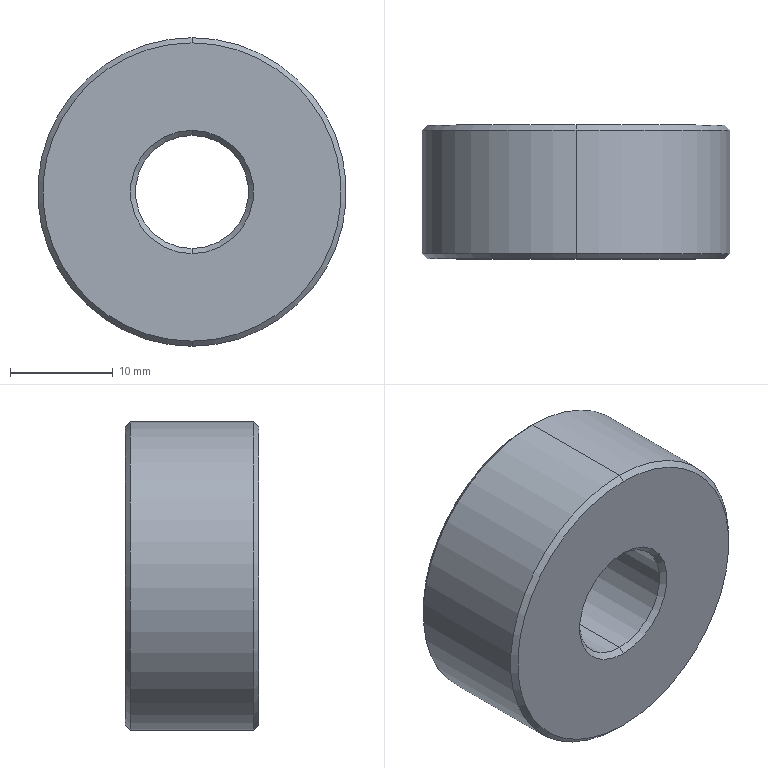Part | STEP file | OP10-032_collar | 1 solid | 14 faces | box 30 x 13 x 30 mm | volume 7922 mm3 | cone 8 | cylinder 4 | plane 2 | commonest cylinder face diameters 11 x2 30 x2
STEP:
#1=CARTESIAN_POINT('',(0.,0.,0.));
#2=DIRECTION('',(0.,0.,1.));
#3=DIRECTION('',(1.,0.,0.));
#4=AXIS2_PLACEMENT_3D('',#1,#2,#3);
#5=CARTESIAN_POINT('',(0.,13.,14.5));
#6=VERTEX_POINT('',#5);
#7=CARTESIAN_POINT('',(0.,13.,-14.5));
#8=VERTEX_POINT('',#7);
#9=CARTESIAN_POINT('',(0.,13.,0.));
#10=DIRECTION('',(0.,1.,0.));
#11=DIRECTION('',(0.,0.,1.));
#12=AXIS2_PLACEMENT_3D('',#9,#10,#11);
#13=CIRCLE('',#12,14.5);
#14=CARTESIAN_POINT('',(0.,13.,0.));
#15=DIRECTION('',(0.,-1.,0.));
#16=DIRECTION('',(0.,0.,-1.));
#17=AXIS2_PLACEMENT_3D('',#14,#15,#16);
#18=CONICAL_SURFACE('',#17,14.5,0.7854);
#19=CARTESIAN_POINT('',(3.142,0.));
#20=DIRECTION('',(-1.,0.));
#21=VECTOR('',#20,1.);
#22=LINE('',#19,#21);
#23=(GEOMETRIC_REPRESENTATION_CONTEXT(2)PARAMETRIC_REPRESENTATION_CONTEXT()REPRESENTATION_CONTEXT('',''));
#24=DEFINITIONAL_REPRESENTATION('',(#22),#23);
#25=PCURVE('',#18,#24);
#26=CARTESIAN_POINT('',(0.,13.,0.));
#27=DIRECTION('',(0.,1.,0.));
#28=DIRECTION('',(0.,0.,1.));
#29=AXIS2_PLACEMENT_3D('',#26,#27,#28);
#30=PLANE('',#29);
#31=CARTESIAN_POINT('',(0.,0.));
#32=DIRECTION('',(1.,0.));
#33=AXIS2_PLACEMENT_2D('',#31,#32);
#34=CIRCLE('',#33,14.5);
#35=(GEOMETRIC_REPRESENTATION_CONTEXT(2)PARAMETRIC_REPRESENTATION_CONTEXT()REPRESENTATION_CONTEXT('',''));
#36=DEFINITIONAL_REPRESENTATION('',(#34),#35);
#37=PCURVE('',#30,#36);
#38=SURFACE_CURVE('',#13,(#25,#37),.PCURVE_S1.);
#39=EDGE_CURVE('',#6,#8,#38,.T.);
#40=ORIENTED_EDGE('',*,*,#39,.F.);
#41=CARTESIAN_POINT('',(0.,12.5,15.));
#42=VERTEX_POINT('',#41);
#43=CARTESIAN_POINT('',(0.,13.,14.5));
#44=DIRECTION('',(0.,-0.7071,0.7071));
#45=VECTOR('',#44,1.);
#46=LINE('',#43,#45);
#47=CARTESIAN_POINT('',(3.142,0.));
#48=DIRECTION('',(0.,1.));
#49=VECTOR('',#48,1.);
#50=LINE('',#47,#49);
#51=(GEOMETRIC_REPRESENTATION_CONTEXT(2)PARAMETRIC_REPRESENTATION_CONTEXT()REPRESENTATION_CONTEXT('',''));
#52=DEFINITIONAL_REPRESENTATION('',(#50),#51);
#53=PCURVE('',#18,#52);
#54=CARTESIAN_POINT('',(0.,13.,0.));
#55=DIRECTION('',(0.,-1.,0.));
#56=DIRECTION('',(0.,0.,-1.));
#57=AXIS2_PLACEMENT_3D('',#54,#55,#56);
#58=CONICAL_SURFACE('',#57,14.5,0.7854);
#59=CARTESIAN_POINT('',(3.142,0.));
#60=DIRECTION('',(0.,1.));
#61=VECTOR('',#60,1.);
#62=LINE('',#59,#61);
#63=(GEOMETRIC_REPRESENTATION_CONTEXT(2)PARAMETRIC_REPRESENTATION_CONTEXT()REPRESENTATION_CONTEXT('',''));
#64=DEFINITIONAL_REPRESENTATION('',(#62),#63);
#65=PCURVE('',#58,#64);
#66=SURFACE_CURVE('',#46,(#53,#65),.PCURVE_S1.);
#67=EDGE_CURVE('',#6,#42,#66,.T.);
#68=ORIENTED_EDGE('',*,*,#67,.T.);
#69=CARTESIAN_POINT('',(0.,12.5,-15.));
#70=VERTEX_POINT('',#69);
#71=CARTESIAN_POINT('',(0.,12.5,0.));
#72=DIRECTION('',(0.,-1.,0.));
#73=DIRECTION('',(0.,0.,1.));
#74=AXIS2_PLACEMENT_3D('',#71,#72,#73);
#75=CIRCLE('',#74,15.);
#76=CARTESIAN_POINT('',(-3.142,0.5));
#77=DIRECTION('',(1.,0.));
#78=VECTOR('',#77,1.);
#79=LINE('',#76,#78);
#80=(GEOMETRIC_REPRESENTATION_CONTEXT(2)PARAMETRIC_REPRESENTATION_CONTEXT()REPRESENTATION_CONTEXT('',''));
#81=DEFINITIONAL_REPRESENTATION('',(#79),#80);
#82=PCURVE('',#18,#81);
#83=CARTESIAN_POINT('',(0.,13.,0.));
#84=DIRECTION('',(0.,-1.,0.));
#85=DIRECTION('',(0.,0.,-1.));
#86=AXIS2_PLACEMENT_3D('',#83,#84,#85);
#87=CYLINDRICAL_SURFACE('',#86,15.);
#88=CARTESIAN_POINT('',(-3.142,0.5));
#89=DIRECTION('',(1.,0.));
#90=VECTOR('',#89,1.);
#91=LINE('',#88,#90);
#92=(GEOMETRIC_REPRESENTATION_CONTEXT(2)PARAMETRIC_REPRESENTATION_CONTEXT()REPRESENTATION_CONTEXT('',''));
#93=DEFINITIONAL_REPRESENTATION('',(#91),#92);
#94=PCURVE('',#87,#93);
#95=SURFACE_CURVE('',#75,(#82,#94),.PCURVE_S1.);
#96=EDGE_CURVE('',#70,#42,#95,.T.);
#97=ORIENTED_EDGE('',*,*,#96,.F.);
#98=CARTESIAN_POINT('',(0.,13.,-14.5));
#99=DIRECTION('',(0.,-0.7071,-0.7071));
#100=VECTOR('',#99,1.);
#101=LINE('',#98,#100);
#102=CARTESIAN_POINT('',(0.,0.));
#103=DIRECTION('',(0.,1.));
#104=VECTOR('',#103,1.);
#105=LINE('',#102,#104);
#106=(GEOMETRIC_REPRESENTATION_CONTEXT(2)PARAMETRIC_REPRESENTATION_CONTEXT()REPRESENTATION_CONTEXT('',''));
#107=DEFINITIONAL_REPRESENTATION('',(#105),#106);
#108=PCURVE('',#18,#107);
#109=CARTESIAN_POINT('',(6.283,0.));
#110=DIRECTION('',(0.,1.));
#111=VECTOR('',#110,1.);
#112=LINE('',#109,#111);
#113=(GEOMETRIC_REPRESENTATION_CONTEXT(2)PARAMETRIC_REPRESENTATION_CONTEXT()REPRESENTATION_CONTEXT('',''));
#114=DEFINITIONAL_REPRESENTATION('',(#112),#113);
#115=PCURVE('',#58,#114);
#116=SURFACE_CURVE('',#101,(#108,#115),.PCURVE_S1.);
#117=EDGE_CURVE('',#8,#70,#116,.T.);
#118=ORIENTED_EDGE('',*,*,#117,.F.);
#119=EDGE_LOOP('',(#40,#68,#97,#118));
#120=FACE_BOUND('',#119,.T.);
#121=ADVANCED_FACE('',(#120),#18,.T.);
#122=CARTESIAN_POINT('',(0.,12.5,5.5));
#123=VERTEX_POINT('',#122);
#124=CARTESIAN_POINT('',(0.,13.,6.));
#125=VERTEX_POINT('',#124);
#126=CARTESIAN_POINT('',(0.,12.5,5.5));
#127=DIRECTION('',(0.,0.7071,0.7071));
#128=VECTOR('',#127,1.);
#129=LINE('',#126,#128);
#130=CARTESIAN_POINT('',(0.,12.5,0.));
#131=DIRECTION('',(0.,1.,0.));
#132=DIRECTION('',(0.,0.,1.));
#133=AXIS2_PLACEMENT_3D('',#130,#131,#132);
#134=CONICAL_SURFACE('',#133,5.5,0.7854);
#135=CARTESIAN_POINT('',(6.283,0.));
#136=DIRECTION('',(0.,1.));
#137=VECTOR('',#136,1.);
#138=LINE('',#135,#137);
#139=(GEOMETRIC_REPRESENTATION_CONTEXT(2)PARAMETRIC_REPRESENTATION_CONTEXT()REPRESENTATION_CONTEXT('',''));
#140=DEFINITIONAL_REPRESENTATION('',(#138),#139);
#141=PCURVE('',#134,#140);
#142=CARTESIAN_POINT('',(0.,12.5,0.));
#143=DIRECTION('',(0.,1.,0.));
#144=DIRECTION('',(0.,0.,1.));
#145=AXIS2_PLACEMENT_3D('',#142,#143,#144);
#146=CONICAL_SURFACE('',#145,5.5,0.7854);
#147=CARTESIAN_POINT('',(0.,0.));
#148=DIRECTION('',(0.,1.));
#149=VECTOR('',#148,1.);
#150=LINE('',#147,#149);
#151=(GEOMETRIC_REPRESENTATION_CONTEXT(2)PARAMETRIC_REPRESENTATION_CONTEXT()REPRESENTATION_CONTEXT('',''));
#152=DEFINITIONAL_REPRESENTATION('',(#150),#151);
#153=PCURVE('',#146,#152);
#154=SURFACE_CURVE('',#129,(#141,#153),.PCURVE_S1.);
#155=EDGE_CURVE('',#123,#125,#154,.T.);
#156=ORIENTED_EDGE('',*,*,#155,.T.);
#157=CARTESIAN_POINT('',(0.,13.,-6.));
#158=VERTEX_POINT('',#157);
#159=CARTESIAN_POINT('',(0.,13.,0.));
#160=DIRECTION('',(0.,-1.,0.));
#161=DIRECTION('',(0.,0.,1.));
#162=AXIS2_PLACEMENT_3D('',#159,#160,#161);
#163=CIRCLE('',#162,6.);
#164=CARTESIAN_POINT('',(6.283,0.5));
#165=DIRECTION('',(-1.,0.));
#166=VECTOR('',#165,1.);
#167=LINE('',#164,#166);
#168=(GEOMETRIC_REPRESENTATION_CONTEXT(2)PARAMETRIC_REPRESENTATION_CONTEXT()REPRESENTATION_CONTEXT('',''));
#169=DEFINITIONAL_REPRESENTATION('',(#167),#168);
#170=PCURVE('',#134,#169);
#171=CARTESIAN_POINT('',(6.,0.));
#172=CARTESIAN_POINT('',(6.,-10.392));
#173=CARTESIAN_POINT('',(-3.,-5.196));
#174=CARTESIAN_POINT('',(-12.,0.));
#175=CARTESIAN_POINT('',(-3.,5.196));
#176=CARTESIAN_POINT('',(6.,10.392));
#177=CARTESIAN_POINT('',(6.,0.));
#178=(BOUNDED_CURVE()B_SPLINE_CURVE(2,(#171,#172,#173,#174,#175,#176,#177),.UNSPECIFIED.,.T.,.F.)B_SPLINE_CURVE_WITH_KNOTS((1,2,2,2,2,1),(-2.094,0.,2.094,4.189,6.283,8.378),.UNSPECIFIED.)CURVE()GEOMETRIC_REPRESENTATION_ITEM()RATIONAL_B_SPLINE_CURVE((1.,0.5,1.,0.5,1.,0.5,1.))REPRESENTATION_ITEM(''));
#179=(GEOMETRIC_REPRESENTATION_CONTEXT(2)PARAMETRIC_REPRESENTATION_CONTEXT()REPRESENTATION_CONTEXT('',''));
#180=DEFINITIONAL_REPRESENTATION('',(#178),#179);
#181=PCURVE('',#30,#180);
#182=SURFACE_CURVE('',#163,(#170,#181),.PCURVE_S1.);
#183=EDGE_CURVE('',#125,#158,#182,.T.);
#184=ORIENTED_EDGE('',*,*,#183,.T.);
#185=CARTESIAN_POINT('',(0.,12.5,-5.5));
#186=VERTEX_POINT('',#185);
#187=CARTESIAN_POINT('',(0.,12.5,-5.5));
#188=DIRECTION('',(0.,0.7071,-0.7071));
#189=VECTOR('',#188,1.);
#190=LINE('',#187,#189);
#191=CARTESIAN_POINT('',(3.142,0.));
#192=DIRECTION('',(0.,1.));
#193=VECTOR('',#192,1.);
#194=LINE('',#191,#193);
#195=(GEOMETRIC_REPRESENTATION_CONTEXT(2)PARAMETRIC_REPRESENTATION_CONTEXT()REPRESENTATION_CONTEXT('',''));
#196=DEFINITIONAL_REPRESENTATION('',(#194),#195);
#197=PCURVE('',#134,#196);
#198=CARTESIAN_POINT('',(3.142,0.));
#199=DIRECTION('',(0.,1.));
#200=VECTOR('',#199,1.);
#201=LINE('',#198,#200);
#202=(GEOMETRIC_REPRESENTATION_CONTEXT(2)PARAMETRIC_REPRESENTATION_CONTEXT()REPRESENTATION_CONTEXT('',''));
#203=DEFINITIONAL_REPRESENTATION('',(#201),#202);
#204=PCURVE('',#146,#203);
#205=SURFACE_CURVE('',#190,(#197,#204),.PCURVE_S1.);
#206=EDGE_CURVE('',#186,#158,#205,.T.);
#207=ORIENTED_EDGE('',*,*,#206,.F.);
#208=CARTESIAN_POINT('',(0.,12.5,0.));
#209=DIRECTION('',(0.,1.,0.));
#210=DIRECTION('',(0.,0.,1.));
#211=AXIS2_PLACEMENT_3D('',#208,#209,#210);
#212=CIRCLE('',#211,5.5);
#213=CARTESIAN_POINT('',(0.,0.));
#214=DIRECTION('',(1.,0.));
#215=VECTOR('',#214,1.);
#216=LINE('',#213,#215);
#217=(GEOMETRIC_REPRESENTATION_CONTEXT(2)PARAMETRIC_REPRESENTATION_CONTEXT()REPRESENTATION_CONTEXT('',''));
#218=DEFINITIONAL_REPRESENTATION('',(#216),#217);
#219=PCURVE('',#134,#218);
#220=CARTESIAN_POINT('',(0.,13.,0.));
#221=DIRECTION('',(0.,-1.,0.));
#222=DIRECTION('',(0.,0.,-1.));
#223=AXIS2_PLACEMENT_3D('',#220,#221,#222);
#224=CYLINDRICAL_SURFACE('',#223,5.5);
#225=CARTESIAN_POINT('',(9.425,0.5));
#226=DIRECTION('',(-1.,0.));
#227=VECTOR('',#226,1.);
#228=LINE('',#225,#227);
#229=(GEOMETRIC_REPRESENTATION_CONTEXT(2)PARAMETRIC_REPRESENTATION_CONTEXT()REPRESENTATION_CONTEXT('',''));
#230=DEFINITIONAL_REPRESENTATION('',(#228),#229);
#231=PCURVE('',#224,#230);
#232=SURFACE_CURVE('',#212,(#219,#231),.PCURVE_S1.);
#233=EDGE_CURVE('',#186,#123,#232,.T.);
#234=ORIENTED_EDGE('',*,*,#233,.T.);
#235=EDGE_LOOP('',(#156,#184,#207,#234));
#236=FACE_BOUND('',#235,.F.);
#237=ADVANCED_FACE('',(#236),#134,.F.);
#238=CARTESIAN_POINT('',(0.,0.,-14.5));
#239=VERTEX_POINT('',#238);
#240=CARTESIAN_POINT('',(0.,0.,14.5));
#241=VERTEX_POINT('',#240);
#242=CARTESIAN_POINT('',(0.,0.,0.));
#243=DIRECTION('',(0.,-1.,0.));
#244=DIRECTION('',(0.,0.,1.));
#245=AXIS2_PLACEMENT_3D('',#242,#243,#244);
#246=CIRCLE('',#245,14.5);
#247=CARTESIAN_POINT('',(0.,0.5,0.));
#248=DIRECTION('',(0.,1.,0.));
#249=DIRECTION('',(0.,0.,1.));
#250=AXIS2_PLACEMENT_3D('',#247,#248,#249);
#251=CONICAL_SURFACE('',#250,15.,0.7854);
#252=CARTESIAN_POINT('',(6.283,-0.5));
#253=DIRECTION('',(-1.,0.));
#254=VECTOR('',#253,1.);
#255=LINE('',#252,#254);
#256=(GEOMETRIC_REPRESENTATION_CONTEXT(2)PARAMETRIC_REPRESENTATION_CONTEXT()REPRESENTATION_CONTEXT('',''));
#257=DEFINITIONAL_REPRESENTATION('',(#255),#256);
#258=PCURVE('',#251,#257);
#259=CARTESIAN_POINT('',(0.,0.,0.));
#260=DIRECTION('',(0.,1.,0.));
#261=DIRECTION('',(0.,0.,1.));
#262=AXIS2_PLACEMENT_3D('',#259,#260,#261);
#263=PLANE('',#262);
#264=CARTESIAN_POINT('',(14.5,0.));
#265=CARTESIAN_POINT('',(14.5,-25.115));
#266=CARTESIAN_POINT('',(-7.25,-12.557));
#267=CARTESIAN_POINT('',(-29.,0.));
#268=CARTESIAN_POINT('',(-7.25,12.557));
#269=CARTESIAN_POINT('',(14.5,25.115));
#270=CARTESIAN_POINT('',(14.5,0.));
#271=(BOUNDED_CURVE()B_SPLINE_CURVE(2,(#264,#265,#266,#267,#268,#269,#270),.UNSPECIFIED.,.T.,.F.)B_SPLINE_CURVE_WITH_KNOTS((1,2,2,2,2,1),(-2.094,0.,2.094,4.189,6.283,8.378),.UNSPECIFIED.)CURVE()GEOMETRIC_REPRESENTATION_ITEM()RATIONAL_B_SPLINE_CURVE((1.,0.5,1.,0.5,1.,0.5,1.))REPRESENTATION_ITEM(''));
#272=(GEOMETRIC_REPRESENTATION_CONTEXT(2)PARAMETRIC_REPRESENTATION_CONTEXT()REPRESENTATION_CONTEXT('',''));
#273=DEFINITIONAL_REPRESENTATION('',(#271),#272);
#274=PCURVE('',#263,#273);
#275=SURFACE_CURVE('',#246,(#258,#274),.PCURVE_S1.);
#276=EDGE_CURVE('',#239,#241,#275,.T.);
#277=ORIENTED_EDGE('',*,*,#276,.F.);
#278=CARTESIAN_POINT('',(0.,0.5,-15.));
#279=VERTEX_POINT('',#278);
#280=CARTESIAN_POINT('',(0.,0.5,-15.));
#281=DIRECTION('',(0.,0.7071,-0.7071));
#282=VECTOR('',#281,1.);
#283=LINE('',#280,#282);
#284=CARTESIAN_POINT('',(3.142,0.));
#285=DIRECTION('',(0.,1.));
#286=VECTOR('',#285,1.);
#287=LINE('',#284,#286);
#288=(GEOMETRIC_REPRESENTATION_CONTEXT(2)PARAMETRIC_REPRESENTATION_CONTEXT()REPRESENTATION_CONTEXT('',''));
#289=DEFINITIONAL_REPRESENTATION('',(#287),#288);
#290=PCURVE('',#251,#289);
#291=CARTESIAN_POINT('',(0.,0.5,0.));
#292=DIRECTION('',(0.,1.,0.));
#293=DIRECTION('',(0.,0.,1.));
#294=AXIS2_PLACEMENT_3D('',#291,#292,#293);
#295=CONICAL_SURFACE('',#294,15.,0.7854);
#296=CARTESIAN_POINT('',(3.142,0.));
#297=DIRECTION('',(0.,1.));
#298=VECTOR('',#297,1.);
#299=LINE('',#296,#298);
#300=(GEOMETRIC_REPRESENTATION_CONTEXT(2)PARAMETRIC_REPRESENTATION_CONTEXT()REPRESENTATION_CONTEXT('',''));
#301=DEFINITIONAL_REPRESENTATION('',(#299),#300);
#302=PCURVE('',#295,#301);
#303=SURFACE_CURVE('',#283,(#290,#302),.PCURVE_S1.);
#304=EDGE_CURVE('',#239,#279,#303,.T.);
#305=ORIENTED_EDGE('',*,*,#304,.T.);
#306=CARTESIAN_POINT('',(0.,0.5,15.));
#307=VERTEX_POINT('',#306);
#308=CARTESIAN_POINT('',(0.,0.5,0.));
#309=DIRECTION('',(0.,1.,0.));
#310=DIRECTION('',(0.,0.,1.));
#311=AXIS2_PLACEMENT_3D('',#308,#309,#310);
#312=CIRCLE('',#311,15.);
#313=CARTESIAN_POINT('',(0.,0.));
#314=DIRECTION('',(1.,0.));
#315=VECTOR('',#314,1.);
#316=LINE('',#313,#315);
#317=(GEOMETRIC_REPRESENTATION_CONTEXT(2)PARAMETRIC_REPRESENTATION_CONTEXT()REPRESENTATION_CONTEXT('',''));
#318=DEFINITIONAL_REPRESENTATION('',(#316),#317);
#319=PCURVE('',#251,#318);
#320=CARTESIAN_POINT('',(3.142,12.5));
#321=DIRECTION('',(-1.,0.));
#322=VECTOR('',#321,1.);
#323=LINE('',#320,#322);
#324=(GEOMETRIC_REPRESENTATION_CONTEXT(2)PARAMETRIC_REPRESENTATION_CONTEXT()REPRESENTATION_CONTEXT('',''));
#325=DEFINITIONAL_REPRESENTATION('',(#323),#324);
#326=PCURVE('',#87,#325);
#327=SURFACE_CURVE('',#312,(#319,#326),.PCURVE_S1.);
#328=EDGE_CURVE('',#307,#279,#327,.T.);
#329=ORIENTED_EDGE('',*,*,#328,.F.);
#330=CARTESIAN_POINT('',(0.,0.5,15.));
#331=DIRECTION('',(0.,0.7071,0.7071));
#332=VECTOR('',#331,1.);
#333=LINE('',#330,#332);
#334=CARTESIAN_POINT('',(0.,0.));
#335=DIRECTION('',(0.,1.));
#336=VECTOR('',#335,1.);
#337=LINE('',#334,#336);
#338=(GEOMETRIC_REPRESENTATION_CONTEXT(2)PARAMETRIC_REPRESENTATION_CONTEXT()REPRESENTATION_CONTEXT('',''));
#339=DEFINITIONAL_REPRESENTATION('',(#337),#338);
#340=PCURVE('',#251,#339);
#341=CARTESIAN_POINT('',(6.283,0.));
#342=DIRECTION('',(0.,1.));
#343=VECTOR('',#342,1.);
#344=LINE('',#341,#343);
#345=(GEOMETRIC_REPRESENTATION_CONTEXT(2)PARAMETRIC_REPRESENTATION_CONTEXT()REPRESENTATION_CONTEXT('',''));
#346=DEFINITIONAL_REPRESENTATION('',(#344),#345);
#347=PCURVE('',#295,#346);
#348=SURFACE_CURVE('',#333,(#340,#347),.PCURVE_S1.);
#349=EDGE_CURVE('',#241,#307,#348,.T.);
#350=ORIENTED_EDGE('',*,*,#349,.F.);
#351=EDGE_LOOP('',(#277,#305,#329,#350));
#352=FACE_BOUND('',#351,.T.);
#353=ADVANCED_FACE('',(#352),#251,.T.);
#354=CARTESIAN_POINT('',(0.,0.5,-5.5));
#355=VERTEX_POINT('',#354);
#356=CARTESIAN_POINT('',(0.,0.,-6.));
#357=VERTEX_POINT('',#356);
#358=CARTESIAN_POINT('',(0.,0.,-6.));
#359=DIRECTION('',(0.,-0.7071,-0.7071));
#360=VECTOR('',#359,1.);
#361=LINE('',#358,#360);
#362=CARTESIAN_POINT('',(0.,0.,0.));
#363=DIRECTION('',(0.,-1.,0.));
#364=DIRECTION('',(0.,0.,-1.));
#365=AXIS2_PLACEMENT_3D('',#362,#363,#364);
#366=CONICAL_SURFACE('',#365,6.,0.7854);
#367=CARTESIAN_POINT('',(6.283,0.));
#368=DIRECTION('',(0.,1.));
#369=VECTOR('',#368,1.);
#370=LINE('',#367,#369);
#371=(GEOMETRIC_REPRESENTATION_CONTEXT(2)PARAMETRIC_REPRESENTATION_CONTEXT()REPRESENTATION_CONTEXT('',''));
#372=DEFINITIONAL_REPRESENTATION('',(#370),#371);
#373=PCURVE('',#366,#372);
#374=CARTESIAN_POINT('',(0.,0.,0.));
#375=DIRECTION('',(0.,-1.,0.));
#376=DIRECTION('',(0.,0.,-1.));
#377=AXIS2_PLACEMENT_3D('',#374,#375,#376);
#378=CONICAL_SURFACE('',#377,6.,0.7854);
#379=CARTESIAN_POINT('',(0.,0.));
#380=DIRECTION('',(0.,1.));
#381=VECTOR('',#380,1.);
#382=LINE('',#379,#381);
#383=(GEOMETRIC_REPRESENTATION_CONTEXT(2)PARAMETRIC_REPRESENTATION_CONTEXT()REPRESENTATION_CONTEXT('',''));
#384=DEFINITIONAL_REPRESENTATION('',(#382),#383);
#385=PCURVE('',#378,#384);
#386=SURFACE_CURVE('',#361,(#373,#385),.PCURVE_S1.);
#387=EDGE_CURVE('',#355,#357,#386,.T.);
#388=ORIENTED_EDGE('',*,*,#387,.T.);
#389=CARTESIAN_POINT('',(0.,0.,6.));
#390=VERTEX_POINT('',#389);
#391=CARTESIAN_POINT('',(0.,0.,0.));
#392=DIRECTION('',(0.,1.,0.));
#393=DIRECTION('',(0.,0.,1.));
#394=AXIS2_PLACEMENT_3D('',#391,#392,#393);
#395=CIRCLE('',#394,6.);
#396=CARTESIAN_POINT('',(9.425,0.));
#397=DIRECTION('',(-1.,0.));
#398=VECTOR('',#397,1.);
#399=LINE('',#396,#398);
#400=(GEOMETRIC_REPRESENTATION_CONTEXT(2)PARAMETRIC_REPRESENTATION_CONTEXT()REPRESENTATION_CONTEXT('',''));
#401=DEFINITIONAL_REPRESENTATION('',(#399),#400);
#402=PCURVE('',#366,#401);
#403=CARTESIAN_POINT('',(0.,0.));
#404=DIRECTION('',(1.,0.));
#405=AXIS2_PLACEMENT_2D('',#403,#404);
#406=CIRCLE('',#405,6.);
#407=(GEOMETRIC_REPRESENTATION_CONTEXT(2)PARAMETRIC_REPRESENTATION_CONTEXT()REPRESENTATION_CONTEXT('',''));
#408=DEFINITIONAL_REPRESENTATION('',(#406),#407);
#409=PCURVE('',#263,#408);
#410=SURFACE_CURVE('',#395,(#402,#409),.PCURVE_S1.);
#411=EDGE_CURVE('',#357,#390,#410,.T.);
#412=ORIENTED_EDGE('',*,*,#411,.T.);
#413=CARTESIAN_POINT('',(0.,0.5,5.5));
#414=VERTEX_POINT('',#413);
#415=CARTESIAN_POINT('',(0.,0.,6.));
#416=DIRECTION('',(0.,-0.7071,0.7071));
#417=VECTOR('',#416,1.);
#418=LINE('',#415,#417);
#419=CARTESIAN_POINT('',(3.142,0.));
#420=DIRECTION('',(0.,1.));
#421=VECTOR('',#420,1.);
#422=LINE('',#419,#421);
#423=(GEOMETRIC_REPRESENTATION_CONTEXT(2)PARAMETRIC_REPRESENTATION_CONTEXT()REPRESENTATION_CONTEXT('',''));
#424=DEFINITIONAL_REPRESENTATION('',(#422),#423);
#425=PCURVE('',#366,#424);
#426=CARTESIAN_POINT('',(3.142,0.));
#427=DIRECTION('',(0.,1.));
#428=VECTOR('',#427,1.);
#429=LINE('',#426,#428);
#430=(GEOMETRIC_REPRESENTATION_CONTEXT(2)PARAMETRIC_REPRESENTATION_CONTEXT()REPRESENTATION_CONTEXT('',''));
#431=DEFINITIONAL_REPRESENTATION('',(#429),#430);
#432=PCURVE('',#378,#431);
#433=SURFACE_CURVE('',#418,(#425,#432),.PCURVE_S1.);
#434=EDGE_CURVE('',#414,#390,#433,.T.);
#435=ORIENTED_EDGE('',*,*,#434,.F.);
#436=CARTESIAN_POINT('',(0.,0.5,0.));
#437=DIRECTION('',(0.,-1.,0.));
#438=DIRECTION('',(0.,0.,1.));
#439=AXIS2_PLACEMENT_3D('',#436,#437,#438);
#440=CIRCLE('',#439,5.5);
#441=CARTESIAN_POINT('',(3.142,-0.5));
#442=DIRECTION('',(1.,0.));
#443=VECTOR('',#442,1.);
#444=LINE('',#441,#443);
#445=(GEOMETRIC_REPRESENTATION_CONTEXT(2)PARAMETRIC_REPRESENTATION_CONTEXT()REPRESENTATION_CONTEXT('',''));
#446=DEFINITIONAL_REPRESENTATION('',(#444),#445);
#447=PCURVE('',#366,#446);
#448=CARTESIAN_POINT('',(3.142,12.5));
#449=DIRECTION('',(1.,0.));
#450=VECTOR('',#449,1.);
#451=LINE('',#448,#450);
#452=(GEOMETRIC_REPRESENTATION_CONTEXT(2)PARAMETRIC_REPRESENTATION_CONTEXT()REPRESENTATION_CONTEXT('',''));
#453=DEFINITIONAL_REPRESENTATION('',(#451),#452);
#454=PCURVE('',#224,#453);
#455=SURFACE_CURVE('',#440,(#447,#454),.PCURVE_S1.);
#456=EDGE_CURVE('',#414,#355,#455,.T.);
#457=ORIENTED_EDGE('',*,*,#456,.T.);
#458=EDGE_LOOP('',(#388,#412,#435,#457));
#459=FACE_BOUND('',#458,.F.);
#460=ADVANCED_FACE('',(#459),#366,.F.);
#461=CARTESIAN_POINT('',(0.,13.,-5.5));
#462=DIRECTION('',(0.,-1.,0.));
#463=VECTOR('',#462,1.);
#464=LINE('',#461,#463);
#465=CARTESIAN_POINT('',(6.283,0.));
#466=DIRECTION('',(0.,1.));
#467=VECTOR('',#466,1.);
#468=LINE('',#465,#467);
#469=(GEOMETRIC_REPRESENTATION_CONTEXT(2)PARAMETRIC_REPRESENTATION_CONTEXT()REPRESENTATION_CONTEXT('',''));
#470=DEFINITIONAL_REPRESENTATION('',(#468),#469);
#471=PCURVE('',#224,#470);
#472=CARTESIAN_POINT('',(0.,13.,0.));
#473=DIRECTION('',(0.,-1.,0.));
#474=DIRECTION('',(0.,0.,-1.));
#475=AXIS2_PLACEMENT_3D('',#472,#473,#474);
#476=CYLINDRICAL_SURFACE('',#475,5.5);
#477=CARTESIAN_POINT('',(0.,0.));
#478=DIRECTION('',(0.,1.));
#479=VECTOR('',#478,1.);
#480=LINE('',#477,#479);
#481=(GEOMETRIC_REPRESENTATION_CONTEXT(2)PARAMETRIC_REPRESENTATION_CONTEXT()REPRESENTATION_CONTEXT('',''));
#482=DEFINITIONAL_REPRESENTATION('',(#480),#481);
#483=PCURVE('',#476,#482);
#484=SURFACE_CURVE('',#464,(#471,#483),.PCURVE_S1.);
#485=EDGE_CURVE('',#186,#355,#484,.T.);
#486=ORIENTED_EDGE('',*,*,#485,.T.);
#487=ORIENTED_EDGE('',*,*,#456,.F.);
#488=CARTESIAN_POINT('',(0.,13.,5.5));
#489=DIRECTION('',(0.,-1.,0.));
#490=VECTOR('',#489,1.);
#491=LINE('',#488,#490);
#492=CARTESIAN_POINT('',(3.142,0.));
#493=DIRECTION('',(0.,1.));
#494=VECTOR('',#493,1.);
#495=LINE('',#492,#494);
#496=(GEOMETRIC_REPRESENTATION_CONTEXT(2)PARAMETRIC_REPRESENTATION_CONTEXT()REPRESENTATION_CONTEXT('',''));
#497=DEFINITIONAL_REPRESENTATION('',(#495),#496);
#498=PCURVE('',#224,#497);
#499=CARTESIAN_POINT('',(3.142,0.));
#500=DIRECTION('',(0.,1.));
#501=VECTOR('',#500,1.);
#502=LINE('',#499,#501);
#503=(GEOMETRIC_REPRESENTATION_CONTEXT(2)PARAMETRIC_REPRESENTATION_CONTEXT()REPRESENTATION_CONTEXT('',''));
#504=DEFINITIONAL_REPRESENTATION('',(#502),#503);
#505=PCURVE('',#476,#504);
#506=SURFACE_CURVE('',#491,(#498,#505),.PCURVE_S1.);
#507=EDGE_CURVE('',#123,#414,#506,.T.);
#508=ORIENTED_EDGE('',*,*,#507,.F.);
#509=ORIENTED_EDGE('',*,*,#233,.F.);
#510=EDGE_LOOP('',(#486,#487,#508,#509));
#511=FACE_BOUND('',#510,.F.);
#512=ADVANCED_FACE('',(#511),#224,.F.);
#513=ORIENTED_EDGE('',*,*,#96,.T.);
#514=CARTESIAN_POINT('',(0.,13.,15.));
#515=DIRECTION('',(0.,-1.,0.));
#516=VECTOR('',#515,1.);
#517=LINE('',#514,#516);
#518=CARTESIAN_POINT('',(3.142,0.));
#519=DIRECTION('',(0.,1.));
#520=VECTOR('',#519,1.);
#521=LINE('',#518,#520);
#522=(GEOMETRIC_REPRESENTATION_CONTEXT(2)PARAMETRIC_REPRESENTATION_CONTEXT()REPRESENTATION_CONTEXT('',''));
#523=DEFINITIONAL_REPRESENTATION('',(#521),#522);
#524=PCURVE('',#87,#523);
#525=CARTESIAN_POINT('',(0.,13.,0.));
#526=DIRECTION('',(0.,-1.,0.));
#527=DIRECTION('',(0.,0.,-1.));
#528=AXIS2_PLACEMENT_3D('',#525,#526,#527);
#529=CYLINDRICAL_SURFACE('',#528,15.);
#530=CARTESIAN_POINT('',(3.142,0.));
#531=DIRECTION('',(0.,1.));
#532=VECTOR('',#531,1.);
#533=LINE('',#530,#532);
#534=(GEOMETRIC_REPRESENTATION_CONTEXT(2)PARAMETRIC_REPRESENTATION_CONTEXT()REPRESENTATION_CONTEXT('',''));
#535=DEFINITIONAL_REPRESENTATION('',(#533),#534);
#536=PCURVE('',#529,#535);
#537=SURFACE_CURVE('',#517,(#524,#536),.PCURVE_S1.);
#538=EDGE_CURVE('',#42,#307,#537,.T.);
#539=ORIENTED_EDGE('',*,*,#538,.T.);
#540=ORIENTED_EDGE('',*,*,#328,.T.);
#541=CARTESIAN_POINT('',(0.,13.,-15.));
#542=DIRECTION('',(0.,-1.,0.));
#543=VECTOR('',#542,1.);
#544=LINE('',#541,#543);
#545=CARTESIAN_POINT('',(0.,0.));
#546=DIRECTION('',(0.,1.));
#547=VECTOR('',#546,1.);
#548=LINE('',#545,#547);
#549=(GEOMETRIC_REPRESENTATION_CONTEXT(2)PARAMETRIC_REPRESENTATION_CONTEXT()REPRESENTATION_CONTEXT('',''));
#550=DEFINITIONAL_REPRESENTATION('',(#548),#549);
#551=PCURVE('',#87,#550);
#552=CARTESIAN_POINT('',(6.283,0.));
#553=DIRECTION('',(0.,1.));
#554=VECTOR('',#553,1.);
#555=LINE('',#552,#554);
#556=(GEOMETRIC_REPRESENTATION_CONTEXT(2)PARAMETRIC_REPRESENTATION_CONTEXT()REPRESENTATION_CONTEXT('',''));
#557=DEFINITIONAL_REPRESENTATION('',(#555),#556);
#558=PCURVE('',#529,#557);
#559=SURFACE_CURVE('',#544,(#551,#558),.PCURVE_S1.);
#560=EDGE_CURVE('',#70,#279,#559,.T.);
#561=ORIENTED_EDGE('',*,*,#560,.F.);
#562=EDGE_LOOP('',(#513,#539,#540,#561));
#563=FACE_BOUND('',#562,.T.);
#564=ADVANCED_FACE('',(#563),#87,.T.);
#565=ORIENTED_EDGE('',*,*,#183,.T.);
#566=CARTESIAN_POINT('',(0.,13.,0.));
#567=DIRECTION('',(0.,-1.,0.));
#568=DIRECTION('',(0.,0.,1.));
#569=AXIS2_PLACEMENT_3D('',#566,#567,#568);
#570=CIRCLE('',#569,6.);
#571=CARTESIAN_POINT('',(6.,0.));
#572=CARTESIAN_POINT('',(6.,-10.392));
#573=CARTESIAN_POINT('',(-3.,-5.196));
#574=CARTESIAN_POINT('',(-12.,0.));
#575=CARTESIAN_POINT('',(-3.,5.196));
#576=CARTESIAN_POINT('',(6.,10.392));
#577=CARTESIAN_POINT('',(6.,0.));
#578=(BOUNDED_CURVE()B_SPLINE_CURVE(2,(#571,#572,#573,#574,#575,#576,#577),.UNSPECIFIED.,.T.,.F.)B_SPLINE_CURVE_WITH_KNOTS((1,2,2,2,2,1),(-2.094,0.,2.094,4.189,6.283,8.378),.UNSPECIFIED.)CURVE()GEOMETRIC_REPRESENTATION_ITEM()RATIONAL_B_SPLINE_CURVE((1.,0.5,1.,0.5,1.,0.5,1.))REPRESENTATION_ITEM(''));
#579=(GEOMETRIC_REPRESENTATION_CONTEXT(2)PARAMETRIC_REPRESENTATION_CONTEXT()REPRESENTATION_CONTEXT('',''));
#580=DEFINITIONAL_REPRESENTATION('',(#578),#579);
#581=PCURVE('',#30,#580);
#582=CARTESIAN_POINT('',(6.283,0.5));
#583=DIRECTION('',(-1.,0.));
#584=VECTOR('',#583,1.);
#585=LINE('',#582,#584);
#586=(GEOMETRIC_REPRESENTATION_CONTEXT(2)PARAMETRIC_REPRESENTATION_CONTEXT()REPRESENTATION_CONTEXT('',''));
#587=DEFINITIONAL_REPRESENTATION('',(#585),#586);
#588=PCURVE('',#146,#587);
#589=SURFACE_CURVE('',#570,(#581,#588),.PCURVE_S1.);
#590=EDGE_CURVE('',#158,#125,#589,.T.);
#591=ORIENTED_EDGE('',*,*,#590,.T.);
#592=EDGE_LOOP('',(#565,#591));
#593=FACE_BOUND('',#592,.T.);
#594=CARTESIAN_POINT('',(0.,13.,0.));
#595=DIRECTION('',(0.,1.,0.));
#596=DIRECTION('',(0.,0.,1.));
#597=AXIS2_PLACEMENT_3D('',#594,#595,#596);
#598=CIRCLE('',#597,14.5);
#599=CARTESIAN_POINT('',(0.,0.));
#600=DIRECTION('',(1.,0.));
#601=AXIS2_PLACEMENT_2D('',#599,#600);
#602=CIRCLE('',#601,14.5);
#603=(GEOMETRIC_REPRESENTATION_CONTEXT(2)PARAMETRIC_REPRESENTATION_CONTEXT()REPRESENTATION_CONTEXT('',''));
#604=DEFINITIONAL_REPRESENTATION('',(#602),#603);
#605=PCURVE('',#30,#604);
#606=CARTESIAN_POINT('',(9.425,0.));
#607=DIRECTION('',(-1.,0.));
#608=VECTOR('',#607,1.);
#609=LINE('',#606,#608);
#610=(GEOMETRIC_REPRESENTATION_CONTEXT(2)PARAMETRIC_REPRESENTATION_CONTEXT()REPRESENTATION_CONTEXT('',''));
#611=DEFINITIONAL_REPRESENTATION('',(#609),#610);
#612=PCURVE('',#58,#611);
#613=SURFACE_CURVE('',#598,(#605,#612),.PCURVE_S1.);
#614=EDGE_CURVE('',#8,#6,#613,.T.);
#615=ORIENTED_EDGE('',*,*,#614,.T.);
#616=ORIENTED_EDGE('',*,*,#39,.T.);
#617=EDGE_LOOP('',(#615,#616));
#618=FACE_BOUND('',#617,.T.);
#619=ADVANCED_FACE('',(#593,#618),#30,.T.);
#620=ORIENTED_EDGE('',*,*,#411,.T.);
#621=CARTESIAN_POINT('',(0.,0.,0.));
#622=DIRECTION('',(0.,1.,0.));
#623=DIRECTION('',(0.,0.,1.));
#624=AXIS2_PLACEMENT_3D('',#621,#622,#623);
#625=CIRCLE('',#624,6.);
#626=CARTESIAN_POINT('',(0.,0.));
#627=DIRECTION('',(1.,0.));
#628=AXIS2_PLACEMENT_2D('',#626,#627);
#629=CIRCLE('',#628,6.);
#630=(GEOMETRIC_REPRESENTATION_CONTEXT(2)PARAMETRIC_REPRESENTATION_CONTEXT()REPRESENTATION_CONTEXT('',''));
#631=DEFINITIONAL_REPRESENTATION('',(#629),#630);
#632=PCURVE('',#263,#631);
#633=CARTESIAN_POINT('',(3.142,0.));
#634=DIRECTION('',(-1.,0.));
#635=VECTOR('',#634,1.);
#636=LINE('',#633,#635);
#637=(GEOMETRIC_REPRESENTATION_CONTEXT(2)PARAMETRIC_REPRESENTATION_CONTEXT()REPRESENTATION_CONTEXT('',''));
#638=DEFINITIONAL_REPRESENTATION('',(#636),#637);
#639=PCURVE('',#378,#638);
#640=SURFACE_CURVE('',#625,(#632,#639),.PCURVE_S1.);
#641=EDGE_CURVE('',#390,#357,#640,.T.);
#642=ORIENTED_EDGE('',*,*,#641,.T.);
#643=EDGE_LOOP('',(#620,#642));
#644=FACE_BOUND('',#643,.T.);
#645=CARTESIAN_POINT('',(0.,0.,0.));
#646=DIRECTION('',(0.,-1.,0.));
#647=DIRECTION('',(0.,0.,1.));
#648=AXIS2_PLACEMENT_3D('',#645,#646,#647);
#649=CIRCLE('',#648,14.5);
#650=CARTESIAN_POINT('',(14.5,0.));
#651=CARTESIAN_POINT('',(14.5,-25.115));
#652=CARTESIAN_POINT('',(-7.25,-12.557));
#653=CARTESIAN_POINT('',(-29.,0.));
#654=CARTESIAN_POINT('',(-7.25,12.557));
#655=CARTESIAN_POINT('',(14.5,25.115));
#656=CARTESIAN_POINT('',(14.5,0.));
#657=(BOUNDED_CURVE()B_SPLINE_CURVE(2,(#650,#651,#652,#653,#654,#655,#656),.UNSPECIFIED.,.T.,.F.)B_SPLINE_CURVE_WITH_KNOTS((1,2,2,2,2,1),(-2.094,0.,2.094,4.189,6.283,8.378),.UNSPECIFIED.)CURVE()GEOMETRIC_REPRESENTATION_ITEM()RATIONAL_B_SPLINE_CURVE((1.,0.5,1.,0.5,1.,0.5,1.))REPRESENTATION_ITEM(''));
#658=(GEOMETRIC_REPRESENTATION_CONTEXT(2)PARAMETRIC_REPRESENTATION_CONTEXT()REPRESENTATION_CONTEXT('',''));
#659=DEFINITIONAL_REPRESENTATION('',(#657),#658);
#660=PCURVE('',#263,#659);
#661=CARTESIAN_POINT('',(6.283,-0.5));
#662=DIRECTION('',(-1.,0.));
#663=VECTOR('',#662,1.);
#664=LINE('',#661,#663);
#665=(GEOMETRIC_REPRESENTATION_CONTEXT(2)PARAMETRIC_REPRESENTATION_CONTEXT()REPRESENTATION_CONTEXT('',''));
#666=DEFINITIONAL_REPRESENTATION('',(#664),#665);
#667=PCURVE('',#295,#666);
#668=SURFACE_CURVE('',#649,(#660,#667),.PCURVE_S1.);
#669=EDGE_CURVE('',#241,#239,#668,.T.);
#670=ORIENTED_EDGE('',*,*,#669,.T.);
#671=ORIENTED_EDGE('',*,*,#276,.T.);
#672=EDGE_LOOP('',(#670,#671));
#673=FACE_BOUND('',#672,.T.);
#674=ADVANCED_FACE('',(#644,#673),#263,.F.);
#675=ORIENTED_EDGE('',*,*,#538,.F.);
#676=CARTESIAN_POINT('',(0.,12.5,0.));
#677=DIRECTION('',(0.,-1.,0.));
#678=DIRECTION('',(0.,0.,1.));
#679=AXIS2_PLACEMENT_3D('',#676,#677,#678);
#680=CIRCLE('',#679,15.);
#681=CARTESIAN_POINT('',(3.142,0.5));
#682=DIRECTION('',(1.,0.));
#683=VECTOR('',#682,1.);
#684=LINE('',#681,#683);
#685=(GEOMETRIC_REPRESENTATION_CONTEXT(2)PARAMETRIC_REPRESENTATION_CONTEXT()REPRESENTATION_CONTEXT('',''));
#686=DEFINITIONAL_REPRESENTATION('',(#684),#685);
#687=PCURVE('',#529,#686);
#688=CARTESIAN_POINT('',(3.142,0.5));
#689=DIRECTION('',(1.,0.));
#690=VECTOR('',#689,1.);
#691=LINE('',#688,#690);
#692=(GEOMETRIC_REPRESENTATION_CONTEXT(2)PARAMETRIC_REPRESENTATION_CONTEXT()REPRESENTATION_CONTEXT('',''));
#693=DEFINITIONAL_REPRESENTATION('',(#691),#692);
#694=PCURVE('',#58,#693);
#695=SURFACE_CURVE('',#680,(#687,#694),.PCURVE_S1.);
#696=EDGE_CURVE('',#42,#70,#695,.T.);
#697=ORIENTED_EDGE('',*,*,#696,.T.);
#698=ORIENTED_EDGE('',*,*,#560,.T.);
#699=CARTESIAN_POINT('',(0.,0.5,0.));
#700=DIRECTION('',(0.,1.,0.));
#701=DIRECTION('',(0.,0.,1.));
#702=AXIS2_PLACEMENT_3D('',#699,#700,#701);
#703=CIRCLE('',#702,15.);
#704=CARTESIAN_POINT('',(9.425,12.5));
#705=DIRECTION('',(-1.,0.));
#706=VECTOR('',#705,1.);
#707=LINE('',#704,#706);
#708=(GEOMETRIC_REPRESENTATION_CONTEXT(2)PARAMETRIC_REPRESENTATION_CONTEXT()REPRESENTATION_CONTEXT('',''));
#709=DEFINITIONAL_REPRESENTATION('',(#707),#708);
#710=PCURVE('',#529,#709);
#711=CARTESIAN_POINT('',(0.,0.));
#712=DIRECTION('',(1.,0.));
#713=VECTOR('',#712,1.);
#714=LINE('',#711,#713);
#715=(GEOMETRIC_REPRESENTATION_CONTEXT(2)PARAMETRIC_REPRESENTATION_CONTEXT()REPRESENTATION_CONTEXT('',''));
#716=DEFINITIONAL_REPRESENTATION('',(#714),#715);
#717=PCURVE('',#295,#716);
#718=SURFACE_CURVE('',#703,(#710,#717),.PCURVE_S1.);
#719=EDGE_CURVE('',#279,#307,#718,.T.);
#720=ORIENTED_EDGE('',*,*,#719,.T.);
#721=EDGE_LOOP('',(#675,#697,#698,#720));
#722=FACE_BOUND('',#721,.T.);
#723=ADVANCED_FACE('',(#722),#529,.T.);
#724=CARTESIAN_POINT('',(0.,0.5,0.));
#725=DIRECTION('',(0.,-1.,0.));
#726=DIRECTION('',(0.,0.,1.));
#727=AXIS2_PLACEMENT_3D('',#724,#725,#726);
#728=CIRCLE('',#727,5.5);
#729=CARTESIAN_POINT('',(-3.142,12.5));
#730=DIRECTION('',(1.,0.));
#731=VECTOR('',#730,1.);
#732=LINE('',#729,#731);
#733=(GEOMETRIC_REPRESENTATION_CONTEXT(2)PARAMETRIC_REPRESENTATION_CONTEXT()REPRESENTATION_CONTEXT('',''));
#734=DEFINITIONAL_REPRESENTATION('',(#732),#733);
#735=PCURVE('',#476,#734);
#736=CARTESIAN_POINT('',(-3.142,-0.5));
#737=DIRECTION('',(1.,0.));
#738=VECTOR('',#737,1.);
#739=LINE('',#736,#738);
#740=(GEOMETRIC_REPRESENTATION_CONTEXT(2)PARAMETRIC_REPRESENTATION_CONTEXT()REPRESENTATION_CONTEXT('',''));
#741=DEFINITIONAL_REPRESENTATION('',(#739),#740);
#742=PCURVE('',#378,#741);
#743=SURFACE_CURVE('',#728,(#735,#742),.PCURVE_S1.);
#744=EDGE_CURVE('',#355,#414,#743,.T.);
#745=ORIENTED_EDGE('',*,*,#744,.F.);
#746=ORIENTED_EDGE('',*,*,#485,.F.);
#747=CARTESIAN_POINT('',(0.,12.5,0.));
#748=DIRECTION('',(0.,1.,0.));
#749=DIRECTION('',(0.,0.,1.));
#750=AXIS2_PLACEMENT_3D('',#747,#748,#749);
#751=CIRCLE('',#750,5.5);
#752=CARTESIAN_POINT('',(3.142,0.5));
#753=DIRECTION('',(-1.,0.));
#754=VECTOR('',#753,1.);
#755=LINE('',#752,#754);
#756=(GEOMETRIC_REPRESENTATION_CONTEXT(2)PARAMETRIC_REPRESENTATION_CONTEXT()REPRESENTATION_CONTEXT('',''));
#757=DEFINITIONAL_REPRESENTATION('',(#755),#756);
#758=PCURVE('',#476,#757);
#759=CARTESIAN_POINT('',(0.,0.));
#760=DIRECTION('',(1.,0.));
#761=VECTOR('',#760,1.);
#762=LINE('',#759,#761);
#763=(GEOMETRIC_REPRESENTATION_CONTEXT(2)PARAMETRIC_REPRESENTATION_CONTEXT()REPRESENTATION_CONTEXT('',''));
#764=DEFINITIONAL_REPRESENTATION('',(#762),#763);
#765=PCURVE('',#146,#764);
#766=SURFACE_CURVE('',#751,(#758,#765),.PCURVE_S1.);
#767=EDGE_CURVE('',#123,#186,#766,.T.);
#768=ORIENTED_EDGE('',*,*,#767,.F.);
#769=ORIENTED_EDGE('',*,*,#507,.T.);
#770=EDGE_LOOP('',(#745,#746,#768,#769));
#771=FACE_BOUND('',#770,.F.);
#772=ADVANCED_FACE('',(#771),#476,.F.);
#773=ORIENTED_EDGE('',*,*,#641,.T.);
#774=ORIENTED_EDGE('',*,*,#387,.F.);
#775=ORIENTED_EDGE('',*,*,#744,.T.);
#776=ORIENTED_EDGE('',*,*,#434,.T.);
#777=EDGE_LOOP('',(#773,#774,#775,#776));
#778=FACE_BOUND('',#777,.F.);
#779=ADVANCED_FACE('',(#778),#378,.F.);
#780=ORIENTED_EDGE('',*,*,#304,.F.);
#781=ORIENTED_EDGE('',*,*,#669,.F.);
#782=ORIENTED_EDGE('',*,*,#349,.T.);
#783=ORIENTED_EDGE('',*,*,#719,.F.);
#784=EDGE_LOOP('',(#780,#781,#782,#783));
#785=FACE_BOUND('',#784,.T.);
#786=ADVANCED_FACE('',(#785),#295,.T.);
#787=ORIENTED_EDGE('',*,*,#590,.T.);
#788=ORIENTED_EDGE('',*,*,#155,.F.);
#789=ORIENTED_EDGE('',*,*,#767,.T.);
#790=ORIENTED_EDGE('',*,*,#206,.T.);
#791=EDGE_LOOP('',(#787,#788,#789,#790));
#792=FACE_BOUND('',#791,.F.);
#793=ADVANCED_FACE('',(#792),#146,.F.);
#794=ORIENTED_EDGE('',*,*,#67,.F.);
#795=ORIENTED_EDGE('',*,*,#614,.F.);
#796=ORIENTED_EDGE('',*,*,#117,.T.);
#797=ORIENTED_EDGE('',*,*,#696,.F.);
#798=EDGE_LOOP('',(#794,#795,#796,#797));
#799=FACE_BOUND('',#798,.T.);
#800=ADVANCED_FACE('',(#799),#58,.T.);
#801=CLOSED_SHELL('',(#121,#237,#353,#460,#512,#564,#619,#674,#723,#772,#779,#786,#793,#800));
#802=MANIFOLD_SOLID_BREP('',#801);
#803=(LENGTH_UNIT()NAMED_UNIT(*)SI_UNIT(.MILLI.,.METRE.));
#804=UNCERTAINTY_MEASURE_WITH_UNIT(LENGTH_MEASURE(0.0000001),#803,'','');
#805=(NAMED_UNIT(*)PLANE_ANGLE_UNIT()SI_UNIT($,.RADIAN.));
#806=(NAMED_UNIT(*)SI_UNIT($,.STERADIAN.)SOLID_ANGLE_UNIT());
#807=(GEOMETRIC_REPRESENTATION_CONTEXT(3)GLOBAL_UNCERTAINTY_ASSIGNED_CONTEXT((#804))GLOBAL_UNIT_ASSIGNED_CONTEXT((#803,#805,#806))REPRESENTATION_CONTEXT('',''));
#808=ADVANCED_BREP_SHAPE_REPRESENTATION('',(#4,#802),#807);